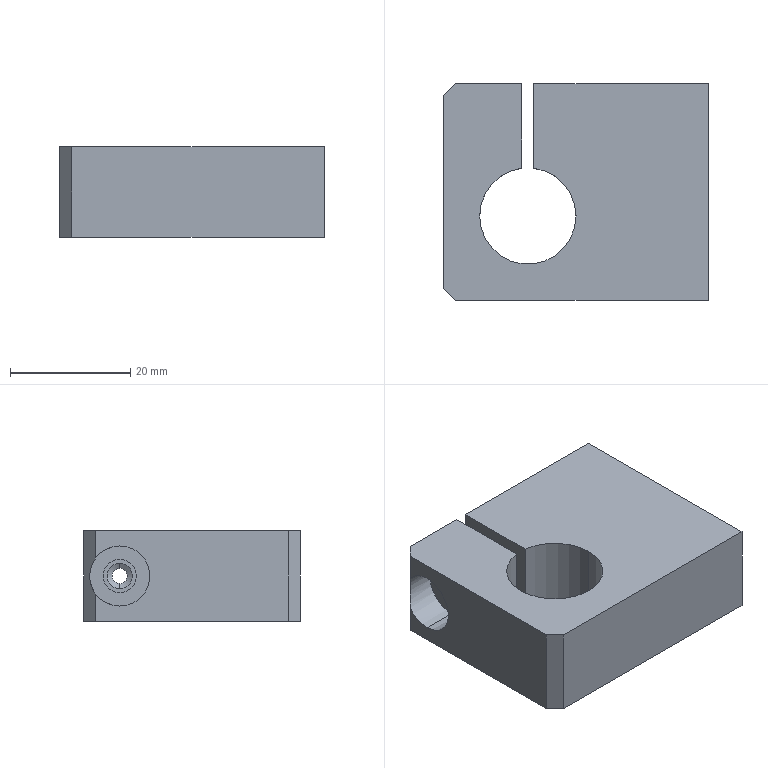Part | STEP file | PN_0106 Mount electronic clip sensor 4 | 1 solid | 31 faces | box 44 x 36 x 15 mm | volume 19047 mm3 | cylinder 13 | plane 12 | cone 6 | commonest cylinder face diameters 4.2 x6 16 x3 5.5 x2 10 x2